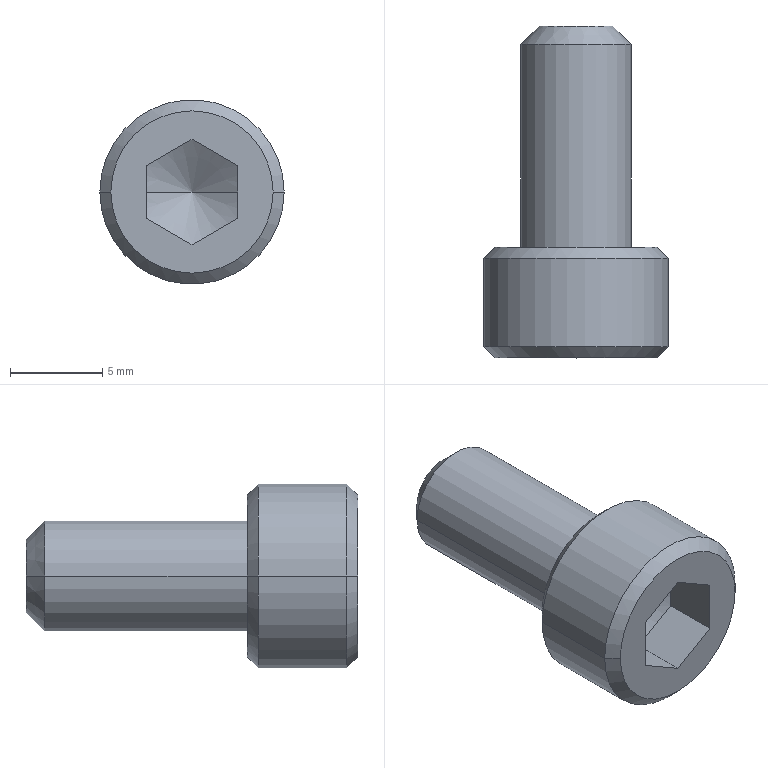Part | STEP file | BB62-M6-12L-2 | 1 solid | 27 faces | box 10 x 18 x 10 mm | volume 713.399 mm3 | plane 15 | cone 8 | cylinder 4 | commonest cylinder face diameters 6 x2 10 x2
STEP:
#1=CARTESIAN_POINT('',(0.,-1.349,0.));
#2=VERTEX_POINT('',#1);
#3=CARTESIAN_POINT('',(2.86,-3.,0.));
#4=VERTEX_POINT('',#3);
#5=CARTESIAN_POINT('',(0.,-1.349,0.));
#6=DIRECTION('',(0.866,-0.5,0.));
#7=VECTOR('',#6,1000.);
#8=LINE('',#5,#7);
#9=EDGE_CURVE('',#2,#4,#8,.T.);
#10=ORIENTED_EDGE('',*,*,#9,.F.);
#11=CARTESIAN_POINT('',(-2.86,-3.,0.));
#12=VERTEX_POINT('',#11);
#13=CARTESIAN_POINT('',(0.,-1.349,0.));
#14=DIRECTION('',(-0.866,-0.5,0.));
#15=VECTOR('',#14,1000.);
#16=LINE('',#13,#15);
#17=EDGE_CURVE('',#2,#12,#16,.T.);
#18=ORIENTED_EDGE('',*,*,#17,.T.);
#19=CARTESIAN_POINT('',(-2.477,-3.,-1.43));
#20=VERTEX_POINT('',#19);
#21=CARTESIAN_POINT('',(0.,-3.,0.));
#22=DIRECTION('',(0.,-1.,0.));
#23=DIRECTION('',(-1.,0.,0.));
#24=AXIS2_PLACEMENT_3D('',#21,#22,#23);
#25=CIRCLE('',#24,2.86);
#26=EDGE_CURVE('',#12,#20,#25,.T.);
#27=ORIENTED_EDGE('',*,*,#26,.T.);
#28=CARTESIAN_POINT('',(0.,-3.,-2.86));
#29=VERTEX_POINT('',#28);
#30=CARTESIAN_POINT('',(0.,-3.,0.));
#31=DIRECTION('',(0.,-1.,0.));
#32=DIRECTION('',(-1.,0.,0.));
#33=AXIS2_PLACEMENT_3D('',#30,#31,#32);
#34=CIRCLE('',#33,2.86);
#35=EDGE_CURVE('',#20,#29,#34,.T.);
#36=ORIENTED_EDGE('',*,*,#35,.T.);
#37=CARTESIAN_POINT('',(2.477,-3.,-1.43));
#38=VERTEX_POINT('',#37);
#39=CARTESIAN_POINT('',(0.,-3.,0.));
#40=DIRECTION('',(0.,-1.,0.));
#41=DIRECTION('',(-1.,0.,0.));
#42=AXIS2_PLACEMENT_3D('',#39,#40,#41);
#43=CIRCLE('',#42,2.86);
#44=EDGE_CURVE('',#29,#38,#43,.T.);
#45=ORIENTED_EDGE('',*,*,#44,.T.);
#46=CARTESIAN_POINT('',(0.,-3.,0.));
#47=DIRECTION('',(0.,-1.,0.));
#48=DIRECTION('',(-1.,0.,0.));
#49=AXIS2_PLACEMENT_3D('',#46,#47,#48);
#50=CIRCLE('',#49,2.86);
#51=EDGE_CURVE('',#38,#4,#50,.T.);
#52=ORIENTED_EDGE('',*,*,#51,.T.);
#53=EDGE_LOOP('',(#10,#18,#27,#36,#45,#52));
#54=FACE_OUTER_BOUND('',#53,.T.);
#55=CARTESIAN_POINT('',(0.,-1001.349,0.));
#56=DIRECTION('',(0.,-1.,0.));
#57=DIRECTION('',(1.,0.,0.));
#58=AXIS2_PLACEMENT_3D('',#55,#56,#57);
#59=CONICAL_SURFACE('',#58,1732.051,1.047);
#60=ADVANCED_FACE('',(#54),#59,.F.);
#61=CARTESIAN_POINT('',(-2.,12.,0.));
#62=VERTEX_POINT('',#61);
#63=CARTESIAN_POINT('',(2.,12.,0.));
#64=VERTEX_POINT('',#63);
#65=CARTESIAN_POINT('',(0.,12.,0.));
#66=DIRECTION('',(0.,1.,0.));
#67=DIRECTION('',(1.,0.,0.));
#68=AXIS2_PLACEMENT_3D('',#65,#66,#67);
#69=CIRCLE('',#68,2.);
#70=EDGE_CURVE('',#62,#64,#69,.T.);
#71=ORIENTED_EDGE('',*,*,#70,.F.);
#72=CARTESIAN_POINT('',(-3.,11.,0.));
#73=VERTEX_POINT('',#72);
#74=CARTESIAN_POINT('',(-2.,12.,0.));
#75=DIRECTION('',(-0.7071,-0.7071,0.));
#76=VECTOR('',#75,1000.);
#77=LINE('',#74,#76);
#78=EDGE_CURVE('',#62,#73,#77,.T.);
#79=ORIENTED_EDGE('',*,*,#78,.T.);
#80=CARTESIAN_POINT('',(3.,11.,0.));
#81=VERTEX_POINT('',#80);
#82=CARTESIAN_POINT('',(0.,11.,0.));
#83=DIRECTION('',(0.,-1.,0.));
#84=DIRECTION('',(-1.,0.,0.));
#85=AXIS2_PLACEMENT_3D('',#82,#83,#84);
#86=CIRCLE('',#85,3.);
#87=EDGE_CURVE('',#81,#73,#86,.T.);
#88=ORIENTED_EDGE('',*,*,#87,.F.);
#89=CARTESIAN_POINT('',(2.,12.,0.));
#90=DIRECTION('',(0.7071,-0.7071,0.));
#91=VECTOR('',#90,1000.);
#92=LINE('',#89,#91);
#93=EDGE_CURVE('',#64,#81,#92,.T.);
#94=ORIENTED_EDGE('',*,*,#93,.F.);
#95=EDGE_LOOP('',(#71,#79,#88,#94));
#96=FACE_OUTER_BOUND('',#95,.T.);
#97=CARTESIAN_POINT('',(0.,12.,0.));
#98=DIRECTION('',(0.,-1.,0.));
#99=DIRECTION('',(1.,0.,0.));
#100=AXIS2_PLACEMENT_3D('',#97,#98,#99);
#101=CONICAL_SURFACE('',#100,2.,0.7854);
#102=ADVANCED_FACE('',(#96),#101,.T.);
#103=ORIENTED_EDGE('',*,*,#87,.T.);
#104=CARTESIAN_POINT('',(-3.,0.,0.));
#105=VERTEX_POINT('',#104);
#106=CARTESIAN_POINT('',(-3.,11.,0.));
#107=DIRECTION('',(0.,-1.,0.));
#108=VECTOR('',#107,1000.);
#109=LINE('',#106,#108);
#110=EDGE_CURVE('',#73,#105,#109,.T.);
#111=ORIENTED_EDGE('',*,*,#110,.T.);
#112=CARTESIAN_POINT('',(3.,0.,0.));
#113=VERTEX_POINT('',#112);
#114=CARTESIAN_POINT('',(0.,0.,0.));
#115=DIRECTION('',(0.,-1.,0.));
#116=DIRECTION('',(-1.,0.,0.));
#117=AXIS2_PLACEMENT_3D('',#114,#115,#116);
#118=CIRCLE('',#117,3.);
#119=EDGE_CURVE('',#113,#105,#118,.T.);
#120=ORIENTED_EDGE('',*,*,#119,.F.);
#121=CARTESIAN_POINT('',(3.,11.,0.));
#122=DIRECTION('',(0.,-1.,0.));
#123=VECTOR('',#122,1000.);
#124=LINE('',#121,#123);
#125=EDGE_CURVE('',#81,#113,#124,.T.);
#126=ORIENTED_EDGE('',*,*,#125,.F.);
#127=EDGE_LOOP('',(#103,#111,#120,#126));
#128=FACE_OUTER_BOUND('',#127,.T.);
#129=CARTESIAN_POINT('',(0.,11.,0.));
#130=DIRECTION('',(0.,-1.,0.));
#131=DIRECTION('',(1.,0.,0.));
#132=AXIS2_PLACEMENT_3D('',#129,#130,#131);
#133=CYLINDRICAL_SURFACE('',#132,3.);
#134=ADVANCED_FACE('',(#128),#133,.T.);
#135=CARTESIAN_POINT('',(4.4,-6.,0.));
#136=VERTEX_POINT('',#135);
#137=CARTESIAN_POINT('',(-4.4,-6.,0.));
#138=VERTEX_POINT('',#137);
#139=CARTESIAN_POINT('',(0.,-6.,0.));
#140=DIRECTION('',(0.,-1.,0.));
#141=DIRECTION('',(-1.,0.,0.));
#142=AXIS2_PLACEMENT_3D('',#139,#140,#141);
#143=CIRCLE('',#142,4.4);
#144=EDGE_CURVE('',#136,#138,#143,.T.);
#145=ORIENTED_EDGE('',*,*,#144,.F.);
#146=CARTESIAN_POINT('',(5.,-5.4,0.));
#147=VERTEX_POINT('',#146);
#148=CARTESIAN_POINT('',(5.,-5.4,0.));
#149=DIRECTION('',(0.7071,0.7071,0.));
#150=VECTOR('',#149,1000.);
#151=LINE('',#148,#150);
#152=EDGE_CURVE('',#136,#147,#151,.T.);
#153=ORIENTED_EDGE('',*,*,#152,.T.);
#154=CARTESIAN_POINT('',(-5.,-5.4,0.));
#155=VERTEX_POINT('',#154);
#156=CARTESIAN_POINT('',(0.,-5.4,0.));
#157=DIRECTION('',(0.,-1.,0.));
#158=DIRECTION('',(-1.,0.,0.));
#159=AXIS2_PLACEMENT_3D('',#156,#157,#158);
#160=CIRCLE('',#159,5.);
#161=EDGE_CURVE('',#147,#155,#160,.T.);
#162=ORIENTED_EDGE('',*,*,#161,.T.);
#163=CARTESIAN_POINT('',(-5.,-5.4,0.));
#164=DIRECTION('',(-0.7071,0.7071,0.));
#165=VECTOR('',#164,1000.);
#166=LINE('',#163,#165);
#167=EDGE_CURVE('',#138,#155,#166,.T.);
#168=ORIENTED_EDGE('',*,*,#167,.F.);
#169=EDGE_LOOP('',(#145,#153,#162,#168));
#170=FACE_OUTER_BOUND('',#169,.T.);
#171=CARTESIAN_POINT('',(0.,-5.4,0.));
#172=DIRECTION('',(0.,1.,0.));
#173=DIRECTION('',(-1.,0.,0.));
#174=AXIS2_PLACEMENT_3D('',#171,#172,#173);
#175=CONICAL_SURFACE('',#174,5.,0.7854);
#176=ADVANCED_FACE('',(#170),#175,.T.);
#177=ORIENTED_EDGE('',*,*,#161,.F.);
#178=CARTESIAN_POINT('',(5.,-0.6,0.));
#179=VERTEX_POINT('',#178);
#180=CARTESIAN_POINT('',(5.,-1.62,0.));
#181=DIRECTION('',(0.,1.,0.));
#182=VECTOR('',#181,1000.);
#183=LINE('',#180,#182);
#184=EDGE_CURVE('',#147,#179,#183,.T.);
#185=ORIENTED_EDGE('',*,*,#184,.T.);
#186=CARTESIAN_POINT('',(-5.,-0.6,0.));
#187=VERTEX_POINT('',#186);
#188=CARTESIAN_POINT('',(0.,-0.6,0.));
#189=DIRECTION('',(0.,-1.,0.));
#190=DIRECTION('',(-1.,0.,0.));
#191=AXIS2_PLACEMENT_3D('',#188,#189,#190);
#192=CIRCLE('',#191,5.);
#193=EDGE_CURVE('',#179,#187,#192,.T.);
#194=ORIENTED_EDGE('',*,*,#193,.T.);
#195=CARTESIAN_POINT('',(-5.,-1.62,0.));
#196=DIRECTION('',(0.,1.,0.));
#197=VECTOR('',#196,1000.);
#198=LINE('',#195,#197);
#199=EDGE_CURVE('',#155,#187,#198,.T.);
#200=ORIENTED_EDGE('',*,*,#199,.F.);
#201=EDGE_LOOP('',(#177,#185,#194,#200));
#202=FACE_OUTER_BOUND('',#201,.T.);
#203=CARTESIAN_POINT('',(0.,-1.62,0.));
#204=DIRECTION('',(0.,1.,0.));
#205=DIRECTION('',(-1.,0.,0.));
#206=AXIS2_PLACEMENT_3D('',#203,#204,#205);
#207=CYLINDRICAL_SURFACE('',#206,5.);
#208=ADVANCED_FACE('',(#202),#207,.T.);
#209=CARTESIAN_POINT('',(4.4,0.,0.));
#210=VERTEX_POINT('',#209);
#211=CARTESIAN_POINT('',(-4.4,0.,0.));
#212=VERTEX_POINT('',#211);
#213=CARTESIAN_POINT('',(0.,0.,0.));
#214=DIRECTION('',(0.,-1.,0.));
#215=DIRECTION('',(-1.,0.,0.));
#216=AXIS2_PLACEMENT_3D('',#213,#214,#215);
#217=CIRCLE('',#216,4.4);
#218=EDGE_CURVE('',#210,#212,#217,.T.);
#219=ORIENTED_EDGE('',*,*,#218,.T.);
#220=CARTESIAN_POINT('',(-4.4,0.,0.));
#221=DIRECTION('',(-0.7071,-0.7071,0.));
#222=VECTOR('',#221,1000.);
#223=LINE('',#220,#222);
#224=EDGE_CURVE('',#212,#187,#223,.T.);
#225=ORIENTED_EDGE('',*,*,#224,.T.);
#226=ORIENTED_EDGE('',*,*,#193,.F.);
#227=CARTESIAN_POINT('',(4.4,0.,0.));
#228=DIRECTION('',(0.7071,-0.7071,0.));
#229=VECTOR('',#228,1000.);
#230=LINE('',#227,#229);
#231=EDGE_CURVE('',#210,#179,#230,.T.);
#232=ORIENTED_EDGE('',*,*,#231,.F.);
#233=EDGE_LOOP('',(#219,#225,#226,#232));
#234=FACE_OUTER_BOUND('',#233,.T.);
#235=CARTESIAN_POINT('',(0.,0.,0.));
#236=DIRECTION('',(0.,-1.,0.));
#237=DIRECTION('',(1.,0.,0.));
#238=AXIS2_PLACEMENT_3D('',#235,#236,#237);
#239=CONICAL_SURFACE('',#238,4.4,0.7854);
#240=ADVANCED_FACE('',(#234),#239,.T.);
#241=CARTESIAN_POINT('',(0.,-6.,0.));
#242=DIRECTION('',(0.,-1.,0.));
#243=DIRECTION('',(-1.,0.,0.));
#244=AXIS2_PLACEMENT_3D('',#241,#242,#243);
#245=CIRCLE('',#244,4.4);
#246=EDGE_CURVE('',#138,#136,#245,.T.);
#247=ORIENTED_EDGE('',*,*,#246,.T.);
#248=ORIENTED_EDGE('',*,*,#144,.T.);
#249=EDGE_LOOP('',(#247,#248));
#250=FACE_OUTER_BOUND('',#249,.T.);
#251=CARTESIAN_POINT('',(0.,-6.,-2.86));
#252=VERTEX_POINT('',#251);
#253=CARTESIAN_POINT('',(-2.477,-6.,-1.43));
#254=VERTEX_POINT('',#253);
#255=CARTESIAN_POINT('',(0.,-6.,-2.86));
#256=DIRECTION('',(-0.866,0.,0.5));
#257=VECTOR('',#256,1000.);
#258=LINE('',#255,#257);
#259=EDGE_CURVE('',#252,#254,#258,.T.);
#260=ORIENTED_EDGE('',*,*,#259,.T.);
#261=CARTESIAN_POINT('',(-2.477,-6.,1.43));
#262=VERTEX_POINT('',#261);
#263=CARTESIAN_POINT('',(-2.477,-6.,-1.43));
#264=DIRECTION('',(0.,0.,1.));
#265=VECTOR('',#264,1000.);
#266=LINE('',#263,#265);
#267=EDGE_CURVE('',#254,#262,#266,.T.);
#268=ORIENTED_EDGE('',*,*,#267,.T.);
#269=CARTESIAN_POINT('',(0.,-6.,2.86));
#270=VERTEX_POINT('',#269);
#271=CARTESIAN_POINT('',(-2.477,-6.,1.43));
#272=DIRECTION('',(0.866,0.,0.5));
#273=VECTOR('',#272,1000.);
#274=LINE('',#271,#273);
#275=EDGE_CURVE('',#262,#270,#274,.T.);
#276=ORIENTED_EDGE('',*,*,#275,.T.);
#277=CARTESIAN_POINT('',(2.477,-6.,1.43));
#278=VERTEX_POINT('',#277);
#279=CARTESIAN_POINT('',(0.,-6.,2.86));
#280=DIRECTION('',(0.866,0.,-0.5));
#281=VECTOR('',#280,1000.);
#282=LINE('',#279,#281);
#283=EDGE_CURVE('',#270,#278,#282,.T.);
#284=ORIENTED_EDGE('',*,*,#283,.T.);
#285=CARTESIAN_POINT('',(2.477,-6.,-1.43));
#286=VERTEX_POINT('',#285);
#287=CARTESIAN_POINT('',(2.477,-6.,1.43));
#288=DIRECTION('',(0.,0.,-1.));
#289=VECTOR('',#288,1000.);
#290=LINE('',#287,#289);
#291=EDGE_CURVE('',#278,#286,#290,.T.);
#292=ORIENTED_EDGE('',*,*,#291,.T.);
#293=CARTESIAN_POINT('',(2.477,-6.,-1.43));
#294=DIRECTION('',(-0.866,0.,-0.5));
#295=VECTOR('',#294,1000.);
#296=LINE('',#293,#295);
#297=EDGE_CURVE('',#286,#252,#296,.T.);
#298=ORIENTED_EDGE('',*,*,#297,.T.);
#299=EDGE_LOOP('',(#260,#268,#276,#284,#292,#298));
#300=FACE_BOUND('',#299,.T.);
#301=CARTESIAN_POINT('',(4.4,-6.,0.));
#302=DIRECTION('',(0.,-1.,0.));
#303=DIRECTION('',(1.,0.,0.));
#304=AXIS2_PLACEMENT_3D('',#301,#302,#303);
#305=PLANE('',#304);
#306=ADVANCED_FACE('',(#250,#300),#305,.T.);
#307=ORIENTED_EDGE('',*,*,#119,.T.);
#308=CARTESIAN_POINT('',(0.,0.,0.));
#309=DIRECTION('',(0.,-1.,0.));
#310=DIRECTION('',(-1.,0.,0.));
#311=AXIS2_PLACEMENT_3D('',#308,#309,#310);
#312=CIRCLE('',#311,3.);
#313=EDGE_CURVE('',#105,#113,#312,.T.);
#314=ORIENTED_EDGE('',*,*,#313,.T.);
#315=EDGE_LOOP('',(#307,#314));
#316=FACE_BOUND('',#315,.T.);
#317=ORIENTED_EDGE('',*,*,#218,.F.);
#318=CARTESIAN_POINT('',(0.,0.,0.));
#319=DIRECTION('',(0.,-1.,0.));
#320=DIRECTION('',(-1.,0.,0.));
#321=AXIS2_PLACEMENT_3D('',#318,#319,#320);
#322=CIRCLE('',#321,4.4);
#323=EDGE_CURVE('',#212,#210,#322,.T.);
#324=ORIENTED_EDGE('',*,*,#323,.F.);
#325=EDGE_LOOP('',(#317,#324));
#326=FACE_OUTER_BOUND('',#325,.T.);
#327=CARTESIAN_POINT('',(0.,0.,0.));
#328=DIRECTION('',(0.,1.,0.));
#329=DIRECTION('',(-1.,0.,0.));
#330=AXIS2_PLACEMENT_3D('',#327,#328,#329);
#331=PLANE('',#330);
#332=ADVANCED_FACE('',(#316,#326),#331,.T.);
#333=ORIENTED_EDGE('',*,*,#224,.F.);
#334=ORIENTED_EDGE('',*,*,#323,.T.);
#335=ORIENTED_EDGE('',*,*,#231,.T.);
#336=CARTESIAN_POINT('',(0.,-0.6,0.));
#337=DIRECTION('',(0.,-1.,0.));
#338=DIRECTION('',(-1.,0.,0.));
#339=AXIS2_PLACEMENT_3D('',#336,#337,#338);
#340=CIRCLE('',#339,5.);
#341=EDGE_CURVE('',#187,#179,#340,.T.);
#342=ORIENTED_EDGE('',*,*,#341,.F.);
#343=EDGE_LOOP('',(#333,#334,#335,#342));
#344=FACE_OUTER_BOUND('',#343,.T.);
#345=CARTESIAN_POINT('',(0.,0.,0.));
#346=DIRECTION('',(0.,-1.,0.));
#347=DIRECTION('',(1.,0.,0.));
#348=AXIS2_PLACEMENT_3D('',#345,#346,#347);
#349=CONICAL_SURFACE('',#348,4.4,0.7854);
#350=ADVANCED_FACE('',(#344),#349,.T.);
#351=ORIENTED_EDGE('',*,*,#184,.F.);
#352=CARTESIAN_POINT('',(0.,-5.4,0.));
#353=DIRECTION('',(0.,-1.,0.));
#354=DIRECTION('',(-1.,0.,0.));
#355=AXIS2_PLACEMENT_3D('',#352,#353,#354);
#356=CIRCLE('',#355,5.);
#357=EDGE_CURVE('',#155,#147,#356,.T.);
#358=ORIENTED_EDGE('',*,*,#357,.F.);
#359=ORIENTED_EDGE('',*,*,#199,.T.);
#360=ORIENTED_EDGE('',*,*,#341,.T.);
#361=EDGE_LOOP('',(#351,#358,#359,#360));
#362=FACE_OUTER_BOUND('',#361,.T.);
#363=CARTESIAN_POINT('',(0.,-1.62,0.));
#364=DIRECTION('',(0.,1.,0.));
#365=DIRECTION('',(-1.,0.,0.));
#366=AXIS2_PLACEMENT_3D('',#363,#364,#365);
#367=CYLINDRICAL_SURFACE('',#366,5.);
#368=ADVANCED_FACE('',(#362),#367,.T.);
#369=ORIENTED_EDGE('',*,*,#152,.F.);
#370=ORIENTED_EDGE('',*,*,#246,.F.);
#371=ORIENTED_EDGE('',*,*,#167,.T.);
#372=ORIENTED_EDGE('',*,*,#357,.T.);
#373=EDGE_LOOP('',(#369,#370,#371,#372));
#374=FACE_OUTER_BOUND('',#373,.T.);
#375=CARTESIAN_POINT('',(0.,-5.4,0.));
#376=DIRECTION('',(0.,1.,0.));
#377=DIRECTION('',(-1.,0.,0.));
#378=AXIS2_PLACEMENT_3D('',#375,#376,#377);
#379=CONICAL_SURFACE('',#378,5.,0.7854);
#380=ADVANCED_FACE('',(#374),#379,.T.);
#381=ORIENTED_EDGE('',*,*,#110,.F.);
#382=CARTESIAN_POINT('',(0.,11.,0.));
#383=DIRECTION('',(0.,-1.,0.));
#384=DIRECTION('',(-1.,0.,0.));
#385=AXIS2_PLACEMENT_3D('',#382,#383,#384);
#386=CIRCLE('',#385,3.);
#387=EDGE_CURVE('',#73,#81,#386,.T.);
#388=ORIENTED_EDGE('',*,*,#387,.T.);
#389=ORIENTED_EDGE('',*,*,#125,.T.);
#390=ORIENTED_EDGE('',*,*,#313,.F.);
#391=EDGE_LOOP('',(#381,#388,#389,#390));
#392=FACE_OUTER_BOUND('',#391,.T.);
#393=CARTESIAN_POINT('',(0.,11.,0.));
#394=DIRECTION('',(0.,-1.,0.));
#395=DIRECTION('',(1.,0.,0.));
#396=AXIS2_PLACEMENT_3D('',#393,#394,#395);
#397=CYLINDRICAL_SURFACE('',#396,3.);
#398=ADVANCED_FACE('',(#392),#397,.T.);
#399=CARTESIAN_POINT('',(0.,12.,0.));
#400=DIRECTION('',(0.,1.,0.));
#401=DIRECTION('',(1.,0.,0.));
#402=AXIS2_PLACEMENT_3D('',#399,#400,#401);
#403=CIRCLE('',#402,2.);
#404=EDGE_CURVE('',#64,#62,#403,.T.);
#405=ORIENTED_EDGE('',*,*,#404,.T.);
#406=ORIENTED_EDGE('',*,*,#70,.T.);
#407=EDGE_LOOP('',(#405,#406));
#408=FACE_OUTER_BOUND('',#407,.T.);
#409=CARTESIAN_POINT('',(0.,12.,0.));
#410=DIRECTION('',(0.,1.,0.));
#411=DIRECTION('',(-1.,0.,0.));
#412=AXIS2_PLACEMENT_3D('',#409,#410,#411);
#413=PLANE('',#412);
#414=ADVANCED_FACE('',(#408),#413,.T.);
#415=ORIENTED_EDGE('',*,*,#78,.F.);
#416=ORIENTED_EDGE('',*,*,#404,.F.);
#417=ORIENTED_EDGE('',*,*,#93,.T.);
#418=ORIENTED_EDGE('',*,*,#387,.F.);
#419=EDGE_LOOP('',(#415,#416,#417,#418));
#420=FACE_OUTER_BOUND('',#419,.T.);
#421=CARTESIAN_POINT('',(0.,12.,0.));
#422=DIRECTION('',(0.,-1.,0.));
#423=DIRECTION('',(1.,0.,0.));
#424=AXIS2_PLACEMENT_3D('',#421,#422,#423);
#425=CONICAL_SURFACE('',#424,2.,0.7854);
#426=ADVANCED_FACE('',(#420),#425,.T.);
#427=CARTESIAN_POINT('',(2.477,-3.,-1.43));
#428=DIRECTION('',(-0.866,0.,-0.5));
#429=VECTOR('',#428,1000.);
#430=LINE('',#427,#429);
#431=EDGE_CURVE('',#38,#29,#430,.T.);
#432=ORIENTED_EDGE('',*,*,#431,.T.);
#433=CARTESIAN_POINT('',(0.,-6.,-2.86));
#434=DIRECTION('',(0.,1.,0.));
#435=VECTOR('',#434,1000.);
#436=LINE('',#433,#435);
#437=EDGE_CURVE('',#252,#29,#436,.T.);
#438=ORIENTED_EDGE('',*,*,#437,.F.);
#439=ORIENTED_EDGE('',*,*,#297,.F.);
#440=CARTESIAN_POINT('',(2.477,-6.,-1.43));
#441=DIRECTION('',(0.,1.,0.));
#442=VECTOR('',#441,1000.);
#443=LINE('',#440,#442);
#444=EDGE_CURVE('',#286,#38,#443,.T.);
#445=ORIENTED_EDGE('',*,*,#444,.T.);
#446=EDGE_LOOP('',(#432,#438,#439,#445));
#447=FACE_OUTER_BOUND('',#446,.T.);
#448=CARTESIAN_POINT('',(2.477,-6.,-1.43));
#449=DIRECTION('',(-0.5,0.,0.866));
#450=DIRECTION('',(0.866,0.,0.5));
#451=AXIS2_PLACEMENT_3D('',#448,#449,#450);
#452=PLANE('',#451);
#453=ADVANCED_FACE('',(#447),#452,.T.);
#454=CARTESIAN_POINT('',(0.,-3.,-2.86));
#455=DIRECTION('',(-0.866,0.,0.5));
#456=VECTOR('',#455,1000.);
#457=LINE('',#454,#456);
#458=EDGE_CURVE('',#29,#20,#457,.T.);
#459=ORIENTED_EDGE('',*,*,#458,.T.);
#460=CARTESIAN_POINT('',(-2.477,-6.,-1.43));
#461=DIRECTION('',(0.,1.,0.));
#462=VECTOR('',#461,1000.);
#463=LINE('',#460,#462);
#464=EDGE_CURVE('',#254,#20,#463,.T.);
#465=ORIENTED_EDGE('',*,*,#464,.F.);
#466=ORIENTED_EDGE('',*,*,#259,.F.);
#467=ORIENTED_EDGE('',*,*,#437,.T.);
#468=EDGE_LOOP('',(#459,#465,#466,#467));
#469=FACE_OUTER_BOUND('',#468,.T.);
#470=CARTESIAN_POINT('',(0.,-6.,-2.86));
#471=DIRECTION('',(0.5,0.,0.866));
#472=DIRECTION('',(0.866,0.,-0.5));
#473=AXIS2_PLACEMENT_3D('',#470,#471,#472);
#474=PLANE('',#473);
#475=ADVANCED_FACE('',(#469),#474,.T.);
#476=CARTESIAN_POINT('',(-2.477,-3.,1.43));
#477=VERTEX_POINT('',#476);
#478=CARTESIAN_POINT('',(-2.477,-3.,-1.43));
#479=DIRECTION('',(0.,0.,1.));
#480=VECTOR('',#479,1000.);
#481=LINE('',#478,#480);
#482=EDGE_CURVE('',#20,#477,#481,.T.);
#483=ORIENTED_EDGE('',*,*,#482,.T.);
#484=CARTESIAN_POINT('',(-2.477,-6.,1.43));
#485=DIRECTION('',(0.,1.,0.));
#486=VECTOR('',#485,1000.);
#487=LINE('',#484,#486);
#488=EDGE_CURVE('',#262,#477,#487,.T.);
#489=ORIENTED_EDGE('',*,*,#488,.F.);
#490=ORIENTED_EDGE('',*,*,#267,.F.);
#491=ORIENTED_EDGE('',*,*,#464,.T.);
#492=EDGE_LOOP('',(#483,#489,#490,#491));
#493=FACE_OUTER_BOUND('',#492,.T.);
#494=CARTESIAN_POINT('',(-2.477,-6.,-1.43));
#495=DIRECTION('',(1.,0.,0.));
#496=DIRECTION('',(0.,0.,-1.));
#497=AXIS2_PLACEMENT_3D('',#494,#495,#496);
#498=PLANE('',#497);
#499=ADVANCED_FACE('',(#493),#498,.T.);
#500=CARTESIAN_POINT('',(0.,-3.,2.86));
#501=VERTEX_POINT('',#500);
#502=CARTESIAN_POINT('',(-2.477,-3.,1.43));
#503=DIRECTION('',(0.866,0.,0.5));
#504=VECTOR('',#503,1000.);
#505=LINE('',#502,#504);
#506=EDGE_CURVE('',#477,#501,#505,.T.);
#507=ORIENTED_EDGE('',*,*,#506,.T.);
#508=CARTESIAN_POINT('',(0.,-6.,2.86));
#509=DIRECTION('',(0.,1.,0.));
#510=VECTOR('',#509,1000.);
#511=LINE('',#508,#510);
#512=EDGE_CURVE('',#270,#501,#511,.T.);
#513=ORIENTED_EDGE('',*,*,#512,.F.);
#514=ORIENTED_EDGE('',*,*,#275,.F.);
#515=ORIENTED_EDGE('',*,*,#488,.T.);
#516=EDGE_LOOP('',(#507,#513,#514,#515));
#517=FACE_OUTER_BOUND('',#516,.T.);
#518=CARTESIAN_POINT('',(-2.477,-6.,1.43));
#519=DIRECTION('',(0.5,0.,-0.866));
#520=DIRECTION('',(-0.866,0.,-0.5));
#521=AXIS2_PLACEMENT_3D('',#518,#519,#520);
#522=PLANE('',#521);
#523=ADVANCED_FACE('',(#517),#522,.T.);
#524=CARTESIAN_POINT('',(2.477,-3.,1.43));
#525=VERTEX_POINT('',#524);
#526=CARTESIAN_POINT('',(0.,-3.,2.86));
#527=DIRECTION('',(0.866,0.,-0.5));
#528=VECTOR('',#527,1000.);
#529=LINE('',#526,#528);
#530=EDGE_CURVE('',#501,#525,#529,.T.);
#531=ORIENTED_EDGE('',*,*,#530,.T.);
#532=CARTESIAN_POINT('',(2.477,-6.,1.43));
#533=DIRECTION('',(0.,1.,0.));
#534=VECTOR('',#533,1000.);
#535=LINE('',#532,#534);
#536=EDGE_CURVE('',#278,#525,#535,.T.);
#537=ORIENTED_EDGE('',*,*,#536,.F.);
#538=ORIENTED_EDGE('',*,*,#283,.F.);
#539=ORIENTED_EDGE('',*,*,#512,.T.);
#540=EDGE_LOOP('',(#531,#537,#538,#539));
#541=FACE_OUTER_BOUND('',#540,.T.);
#542=CARTESIAN_POINT('',(0.,-6.,2.86));
#543=DIRECTION('',(-0.5,0.,-0.866));
#544=DIRECTION('',(-0.866,0.,0.5));
#545=AXIS2_PLACEMENT_3D('',#542,#543,#544);
#546=PLANE('',#545);
#547=ADVANCED_FACE('',(#541),#546,.T.);
#548=CARTESIAN_POINT('',(2.477,-3.,1.43));
#549=DIRECTION('',(0.,0.,-1.));
#550=VECTOR('',#549,1000.);
#551=LINE('',#548,#550);
#552=EDGE_CURVE('',#525,#38,#551,.T.);
#553=ORIENTED_EDGE('',*,*,#552,.T.);
#554=ORIENTED_EDGE('',*,*,#444,.F.);
#555=ORIENTED_EDGE('',*,*,#291,.F.);
#556=ORIENTED_EDGE('',*,*,#536,.T.);
#557=EDGE_LOOP('',(#553,#554,#555,#556));
#558=FACE_OUTER_BOUND('',#557,.T.);
#559=CARTESIAN_POINT('',(2.477,-6.,1.43));
#560=DIRECTION('',(-1.,0.,0.));
#561=DIRECTION('',(0.,0.,1.));
#562=AXIS2_PLACEMENT_3D('',#559,#560,#561);
#563=PLANE('',#562);
#564=ADVANCED_FACE('',(#558),#563,.T.);
#565=ORIENTED_EDGE('',*,*,#431,.F.);
#566=ORIENTED_EDGE('',*,*,#44,.F.);
#567=EDGE_LOOP('',(#565,#566));
#568=FACE_OUTER_BOUND('',#567,.T.);
#569=CARTESIAN_POINT('',(0.,-3.,0.));
#570=DIRECTION('',(0.,-1.,0.));
#571=DIRECTION('',(1.,0.,0.));
#572=AXIS2_PLACEMENT_3D('',#569,#570,#571);
#573=PLANE('',#572);
#574=ADVANCED_FACE('',(#568),#573,.F.);
#575=ORIENTED_EDGE('',*,*,#552,.F.);
#576=CARTESIAN_POINT('',(0.,-3.,0.));
#577=DIRECTION('',(0.,-1.,0.));
#578=DIRECTION('',(-1.,0.,0.));
#579=AXIS2_PLACEMENT_3D('',#576,#577,#578);
#580=CIRCLE('',#579,2.86);
#581=EDGE_CURVE('',#4,#525,#580,.T.);
#582=ORIENTED_EDGE('',*,*,#581,.F.);
#583=ORIENTED_EDGE('',*,*,#51,.F.);
#584=EDGE_LOOP('',(#575,#582,#583));
#585=FACE_OUTER_BOUND('',#584,.T.);
#586=CARTESIAN_POINT('',(0.,-3.,0.));
#587=DIRECTION('',(0.,-1.,0.));
#588=DIRECTION('',(1.,0.,0.));
#589=AXIS2_PLACEMENT_3D('',#586,#587,#588);
#590=PLANE('',#589);
#591=ADVANCED_FACE('',(#585),#590,.F.);
#592=ORIENTED_EDGE('',*,*,#530,.F.);
#593=CARTESIAN_POINT('',(0.,-3.,0.));
#594=DIRECTION('',(0.,-1.,0.));
#595=DIRECTION('',(-1.,0.,0.));
#596=AXIS2_PLACEMENT_3D('',#593,#594,#595);
#597=CIRCLE('',#596,2.86);
#598=EDGE_CURVE('',#525,#501,#597,.T.);
#599=ORIENTED_EDGE('',*,*,#598,.F.);
#600=EDGE_LOOP('',(#592,#599));
#601=FACE_OUTER_BOUND('',#600,.T.);
#602=CARTESIAN_POINT('',(0.,-3.,0.));
#603=DIRECTION('',(0.,-1.,0.));
#604=DIRECTION('',(1.,0.,0.));
#605=AXIS2_PLACEMENT_3D('',#602,#603,#604);
#606=PLANE('',#605);
#607=ADVANCED_FACE('',(#601),#606,.F.);
#608=ORIENTED_EDGE('',*,*,#506,.F.);
#609=CARTESIAN_POINT('',(0.,-3.,0.));
#610=DIRECTION('',(0.,-1.,0.));
#611=DIRECTION('',(-1.,0.,0.));
#612=AXIS2_PLACEMENT_3D('',#609,#610,#611);
#613=CIRCLE('',#612,2.86);
#614=EDGE_CURVE('',#501,#477,#613,.T.);
#615=ORIENTED_EDGE('',*,*,#614,.F.);
#616=EDGE_LOOP('',(#608,#615));
#617=FACE_OUTER_BOUND('',#616,.T.);
#618=CARTESIAN_POINT('',(0.,-3.,0.));
#619=DIRECTION('',(0.,-1.,0.));
#620=DIRECTION('',(1.,0.,0.));
#621=AXIS2_PLACEMENT_3D('',#618,#619,#620);
#622=PLANE('',#621);
#623=ADVANCED_FACE('',(#617),#622,.F.);
#624=ORIENTED_EDGE('',*,*,#482,.F.);
#625=ORIENTED_EDGE('',*,*,#26,.F.);
#626=CARTESIAN_POINT('',(0.,-3.,0.));
#627=DIRECTION('',(0.,-1.,0.));
#628=DIRECTION('',(-1.,0.,0.));
#629=AXIS2_PLACEMENT_3D('',#626,#627,#628);
#630=CIRCLE('',#629,2.86);
#631=EDGE_CURVE('',#477,#12,#630,.T.);
#632=ORIENTED_EDGE('',*,*,#631,.F.);
#633=EDGE_LOOP('',(#624,#625,#632));
#634=FACE_OUTER_BOUND('',#633,.T.);
#635=CARTESIAN_POINT('',(0.,-3.,0.));
#636=DIRECTION('',(0.,-1.,0.));
#637=DIRECTION('',(1.,0.,0.));
#638=AXIS2_PLACEMENT_3D('',#635,#636,#637);
#639=PLANE('',#638);
#640=ADVANCED_FACE('',(#634),#639,.F.);
#641=ORIENTED_EDGE('',*,*,#458,.F.);
#642=ORIENTED_EDGE('',*,*,#35,.F.);
#643=EDGE_LOOP('',(#641,#642));
#644=FACE_OUTER_BOUND('',#643,.T.);
#645=CARTESIAN_POINT('',(0.,-3.,0.));
#646=DIRECTION('',(0.,-1.,0.));
#647=DIRECTION('',(1.,0.,0.));
#648=AXIS2_PLACEMENT_3D('',#645,#646,#647);
#649=PLANE('',#648);
#650=ADVANCED_FACE('',(#644),#649,.F.);
#651=ORIENTED_EDGE('',*,*,#17,.F.);
#652=ORIENTED_EDGE('',*,*,#9,.T.);
#653=ORIENTED_EDGE('',*,*,#581,.T.);
#654=ORIENTED_EDGE('',*,*,#598,.T.);
#655=ORIENTED_EDGE('',*,*,#614,.T.);
#656=ORIENTED_EDGE('',*,*,#631,.T.);
#657=EDGE_LOOP('',(#651,#652,#653,#654,#655,#656));
#658=FACE_OUTER_BOUND('',#657,.T.);
#659=CARTESIAN_POINT('',(0.,-1001.349,0.));
#660=DIRECTION('',(0.,-1.,0.));
#661=DIRECTION('',(1.,0.,0.));
#662=AXIS2_PLACEMENT_3D('',#659,#660,#661);
#663=CONICAL_SURFACE('',#662,1732.051,1.047);
#664=ADVANCED_FACE('',(#658),#663,.F.);
#665=CLOSED_SHELL('',(#60,#102,#134,#176,#208,#240,#306,#332,#350,#368,#380,#398,#414,#426,#453,#475,#499,#523,#547,#564,#574,#591,#607,#623,#640,#650,#664));
#666=MANIFOLD_SOLID_BREP('',#665);
#667=CARTESIAN_POINT('',(0.,0.,0.));
#668=DIRECTION('',(0.,0.,1.));
#669=DIRECTION('',(1.,0.,0.));
#670=AXIS2_PLACEMENT_3D('',#667,#668,#669);
#671=(LENGTH_UNIT()NAMED_UNIT(*)SI_UNIT(.MILLI.,.METRE.));
#672=UNCERTAINTY_MEASURE_WITH_UNIT(LENGTH_MEASURE(0.00001),#671,'','');
#673=(NAMED_UNIT(*)PLANE_ANGLE_UNIT()SI_UNIT($,.RADIAN.));
#674=(NAMED_UNIT(*)SI_UNIT($,.STERADIAN.)SOLID_ANGLE_UNIT());
#675=(GEOMETRIC_REPRESENTATION_CONTEXT(3)GLOBAL_UNCERTAINTY_ASSIGNED_CONTEXT((#672))GLOBAL_UNIT_ASSIGNED_CONTEXT((#671,#673,#674))REPRESENTATION_CONTEXT('',''));
#676=ADVANCED_BREP_SHAPE_REPRESENTATION('',(#666,#670),#675);